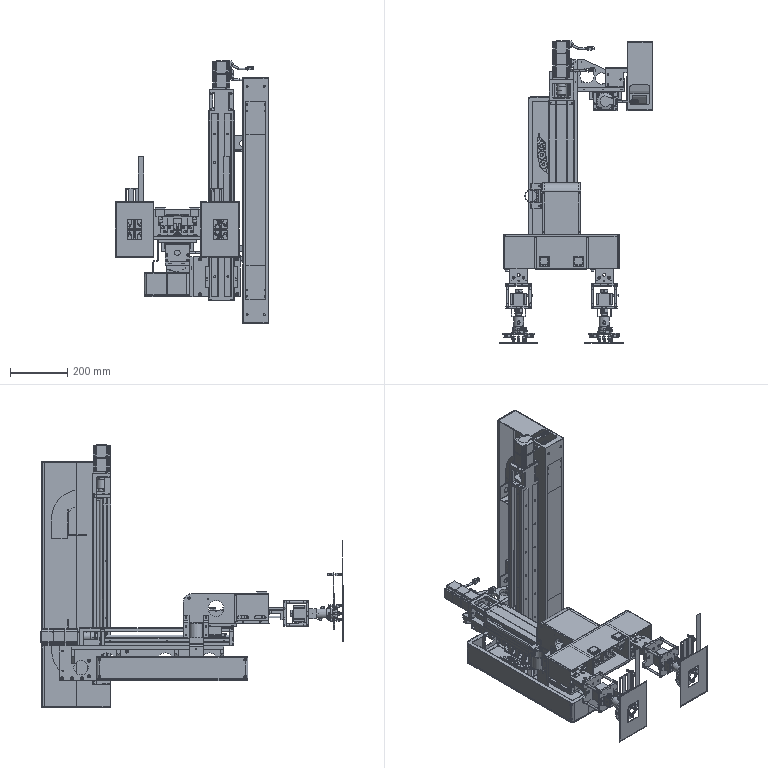Part | NX | 168 solids | 10067 faces | volume 13840906 mm3 | plane 5899 | cylinder 2639 | cone 974 | spline 505 | torus 50 | commonest cylinder face diameters 4 x166 10 x157 8 x136 3.3 x124 5 x124 6 x124